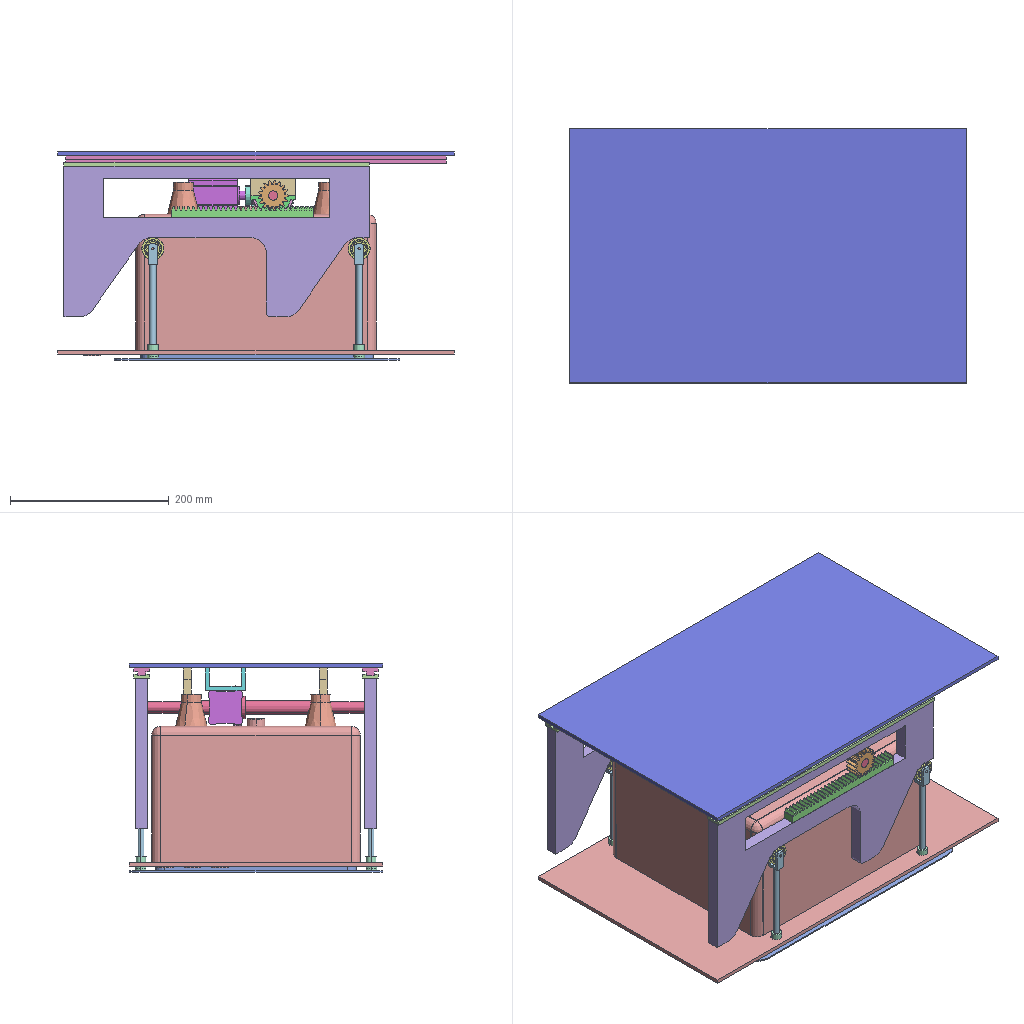Assembly | SolidWorks | 23 different items | 46 placed | box 500 x 320 x 263 mm
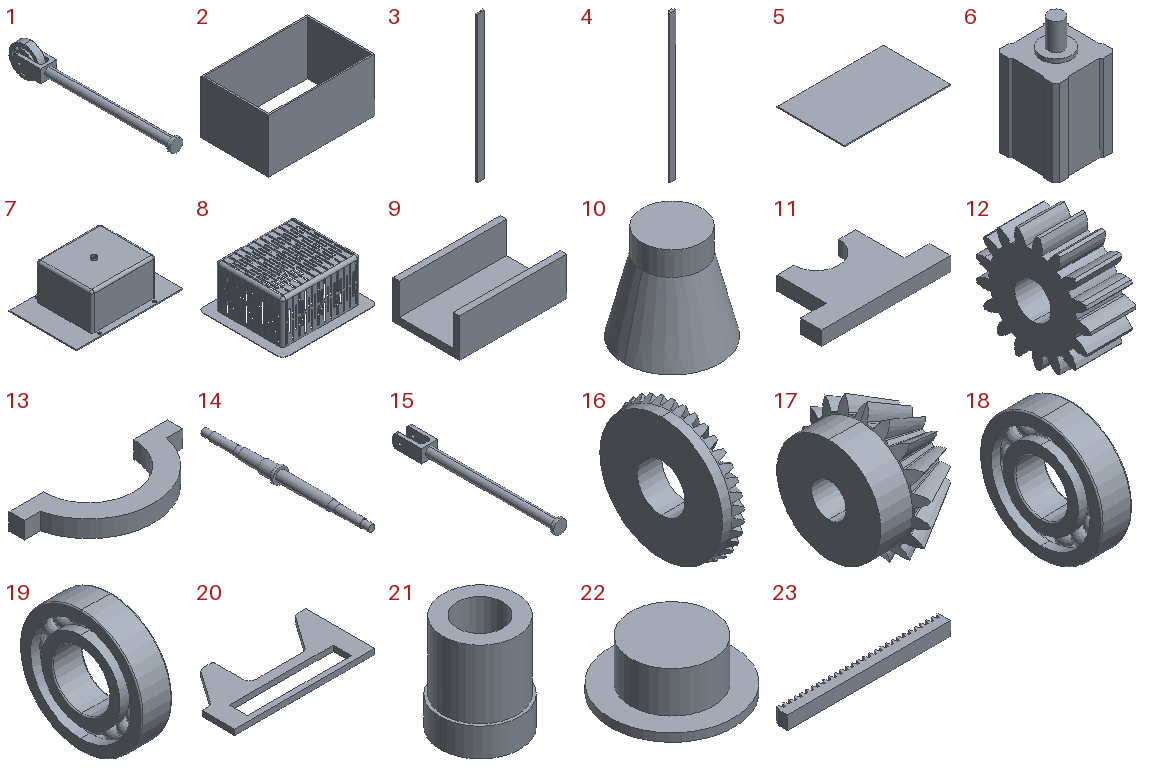Parts list (item | name | quantity | parent item | size | volume | features):
1 | (subassembly) | x4 | - | 15 x 153 x 28 mm | 10997 mm3 | -
2 | - | x1 | - | 500 x 320 x 252.7 mm | 3250733 mm3 | features Extrusion 1
3 | - | x2 | - | 20 x 5 x 385 mm | 30800 mm3 | features Extrusion 1
4 | - | x2 | - | 20 x 10 x 480 mm | 72000 mm3 | features Extrusion 1
5 | - | x1 | - | 500 x 320 x 5 mm | 800000 mm3 | features Extrusion 1
6 | - | x1 | - | 42.35 x 42.35 x 83.6 mm | 106285 mm3 | features ICE 5, CirPattern 1, Extrusion 1, RefAxis 1, Scale 1
7 | - | x1 | - | 500 x 320 x 188.5 mm | 804078 mm3 | features ICE 5, Fillet 2, Extrusion 1
8 | - | x1 | - | 360 x 320 x 163 mm | 306732 mm3 | features ICE 5, Fillet 3, Extrusion 1
9 | - | x1 | - | 80 x 50 x 28.83 mm | 39671 mm3 | features Extrusion 1, ICE 1
10 | - | x4 | - | 40 x 40 x 40 mm | 30238 mm3 | features Blend 1, ICE 1
11 | - | x2 | - | 92 x 50 x 10 mm | 29379 mm3 | features Extrusion 1
12 | - | x2 | - | 15 x 37.761 x 37.916 mm | 11362 mm3 | features Boss 3, Cut 3, CirPattern 2, Fillet 2, Revolution 1
13 | - | x2 | - | 56 x 22.979 x 6 mm | 2901 mm3 | features Extrusion 1
14 | - | x1 | - | 28 x 303 x 28 mm | 67053 mm3 | features Revolution 1
15 | - | x4 | in 1 | 15 x 145 x 12.163 mm | 8356 mm3 | features ICE 3, Fillet 2, Extrusion 1
16 | - | x1 | - | 12.396 x 54.775 x 54.775 mm | 16791 mm3 | features CirPattern 2, Cut 2, BlendCut 1, Boss 1, ICE 1, Revolution 1
17 | - | x1 | - | 19.27 x 30.102 x 30.566 mm | 6755 mm3 | features CirPattern 2, Cut 2, BlendCut 1, Boss 1, Revolution 1
18 | - | x4 | in 1 | 7 x 28 x 28 mm | 2641 mm3 | features Revolution 3, CirPattern 1, Fillet 1
19 | - | x2 | - | 8 x 32 x 32 mm | 3760 mm3 | features Revolution 3, CirPattern 1, Fillet 1
20 | - | x2 | - | 385 x 190 x 15 mm | 496112 mm3 | features Extrusion 1
21 | - | x4 | - | 14 x 14 x 17 mm | 1508 mm3 | features Extrusion 1, ICE 1
22 | - | x1 | - | 30 x 30 x 12 mm | 4555 mm3 | features Extrusion 1, ICE 1
23 | - | x2 | - | 180 x 14 x 15 mm | 31331 mm3 | features Cut 2, Extrusion 1, LPattern 1
Mates (type | each side: item.copy, entity, surface, feature):
In the top assembly
Concentric | 7.1 face cylinder Boss-Extrude3 | 22.1 face cylinder Boss-Extrude2
Coincident | 7.1 face plane Boss-Extrude3 | 22.1 face plane Boss-Extrude1
Coincident | 7.1 face plane Boss-Extrude1 | 8.1 face plane Boss-Extrude1
DistanceDim | 16.1 face plane Hub | 7.1 face plane Boss-Extrude2
Concentric | 16.1 face cylinder Cut-Extrude2 | 12.1 face cylinder Bore
Concentric | 16.1 face cylinder Cut-Extrude2 | 12.2 face cylinder Bore
DistanceDim | 12.1 face plane Base-Revolve | 7.1 face plane Boss-Extrude2
DistanceDim | 12.2 face plane Base-Revolve | 7.1 face plane Boss-Extrude2
Coincident | 12.1 face plane Base-Revolve | 20.1 face plane Boss-Extrude1
Parallel | 7.1 face plane Boss-Extrude3 | 20.1 face plane Boss-Extrude1
Coincident | 12.2 face plane Base-Revolve | 20.2 face plane Boss-Extrude1
Coincident | 20.1 face plane Boss-Extrude1 | 20.2 face plane Boss-Extrude1
Coincident | 20.1 face plane Boss-Extrude1 | 23.1 face plane Blank | 2 times
Concentric | 7.1 face cylinder Cut-Extrude1 | 15.1 face cylinder Boss-Extrude2
Concentric | 7.1 face cylinder Cut-Extrude1 | 15.2 face cylinder Boss-Extrude2
Parallel | 20.1 face plane Boss-Extrude1 | 15.1 face plane Boss-Extrude1
Coincident | 15.1 face plane Boss-Extrude1 | 15.2 face plane Boss-Extrude1
Concentric | 7.1 face cylinder Cut-Extrude1 | 15.3 face cylinder Boss-Extrude2
Parallel | 20.2 face plane Boss-Extrude1 | 15.4 face plane Boss-Extrude1
Parallel | 20.2 face plane Boss-Extrude1 | 15.3 face plane Boss-Extrude1
Coincident | 20.2 face plane Boss-Extrude1 | 23.2 face plane Blank | 2 times
Concentric | 17.1 face cylinder Bore | 6.1 face cylinder Boss-Extrude1
Concentric | 7.1 face cylinder Cut-Extrude1 | 21.1 face cylinder Boss-Extrude2
Coincident | 7.1 face plane Boss-Extrude1 | 21.1 face plane Boss-Extrude1
Concentric | 7.1 face cylinder Cut-Extrude1 | 21.2 face cylinder Boss-Extrude2
Coincident | 7.1 face plane Boss-Extrude1 | 21.2 face plane Boss-Extrude1
Concentric | 7.1 face cylinder Cut-Extrude1 | 21.3 face cylinder Boss-Extrude2
Coincident | 7.1 face plane Boss-Extrude1 | 21.3 face plane Boss-Extrude1
Concentric | 7.1 face cylinder Cut-Extrude1 | 21.4 face cylinder Boss-Extrude2
Coincident | 7.1 face plane Boss-Extrude1 | 21.4 face plane Boss-Extrude1
Coincident | 23.1 face plane Blank | 23.2 face plane Blank | 2 times
DistanceDim | 6.1 face plane Extrude1 | 17.1 face plane Hub
Parallel | 7.1 face plane Boss-Extrude2 | 6.1 face plane Extrude1
Coincident | 7.1 face plane Boss-Extrude1 | 2.1 face plane Boss-Extrude1 | 2 times
DistanceDim | 8.1 face plane Boss-Extrude2 | 7.1 face plane Boss-Extrude1
DistanceDim | 23.1 face plane Blank | 20.1 face plane Boss-Extrude1
Coincident | 10.1 face plane Boss-Extrude1 | 10.2 face plane Boss-Extrude1
Coincident | 7.1 face plane Boss-Extrude3 | 10.1 face plane Loft1
Coincident | 10.1 face plane Boss-Extrude1 | 10.3 face plane Boss-Extrude1
Coincident | 10.1 face plane Boss-Extrude1 | 10.4 face plane Boss-Extrude1
DistanceDim | 10.3 face cylinder Boss-Extrude1 | 7.1 face plane Boss-Extrude2 | 2 times
DistanceDim | 10.2 face cylinder Boss-Extrude1 | 7.1 face plane Boss-Extrude2 | 2 times
DistanceDim | 10.1 face cylinder Boss-Extrude1 | 7.1 face plane Boss-Extrude2 | 2 times
DistanceDim | 10.4 face cylinder Boss-Extrude1 | 7.1 face plane Boss-Extrude2 | 2 times
Coincident | 7.1 face plane Boss-Extrude1 | 5.1 face plane Boss-Extrude1 | 2 times
Coincident | 5.1 face plane Boss-Extrude1 | 4.1 face plane Boss-Extrude1
Coincident | 4.1 face plane Boss-Extrude1 | 4.2 face plane Boss-Extrude1 | 2 times
DistanceDim | 4.1 face plane Boss-Extrude1 | 20.2 face plane Boss-Extrude1
DistanceDim | 4.1 face plane Boss-Extrude1 | 5.1 face plane Boss-Extrude1
DistanceDim | 4.2 face plane Boss-Extrude1 | 20.1 face plane Boss-Extrude1
Coincident | 20.2 face plane Boss-Extrude1 | 3.1 face plane Boss-Extrude1 | 2 times
Coincident | 3.1 face plane Boss-Extrude1 | 4.1 face plane Boss-Extrude1 | 2 times
Coincident | 20.1 face plane Boss-Extrude1 | 3.2 face plane Boss-Extrude1
Coincident | 3.2 face plane Boss-Extrude1 | 4.2 face plane Boss-Extrude1
Coincident | 3.2 face plane Boss-Extrude1 | 20.1 face plane Boss-Extrude1
Parallel | 6.1 face plane Extrude1 | 5.1 face plane Boss-Extrude1
Coincident | 5.1 face plane Boss-Extrude1 | 9.1 face plane Boss-Extrude1
DistanceDim | 6.1 face plane Extrude1 | 9.1 face plane Boss-Extrude1 | 2 times
DistanceDim | 9.1 face plane Boss-Extrude1 | 6.1 face plane Extrude1
Coincident | 15.3 face plane Boss-Extrude3 | 15.4 face plane Boss-Extrude3
Coincident | 15.1 face plane Boss-Extrude3 | 15.4 face plane Boss-Extrude3
Coincident | 15.1 face plane Boss-Extrude3 | 15.2 face plane Boss-Extrude3
Coincident | 8.1 face plane Boss-Extrude1 | 15.2 face plane Boss-Extrude3
DistanceDim | 4.1 face plane Boss-Extrude1 | 21.3 face plane Boss-Extrude2
Tangent | 20.2 face surface:4009 Boss-Extrude1 | 18.1 face cylinder Revolve3
DistanceDim | 6.1 face cylinder Boss-Extrude1 | 16.1 face plane Hub
DistanceDim | 6.1 face plane Extrude1 | 5.1 face plane Boss-Extrude1
Concentric | 12.1 face cylinder Bore | 14.1 face cylinder Revolve1
Coincident | 12.1 face plane Base-Revolve | 14.1 face plane Revolve1
DistanceDim | 14.1 face cylinder Revolve1 | 5.1 face plane Boss-Extrude1
DistanceDim | 17.1 face plane Hub | 14.1 face cylinder Revolve1
Concentric | 14.1 face cylinder Revolve1 | 11.1 face cylinder Boss-Extrude1
Parallel | 5.1 face plane Boss-Extrude1 | 11.1 face plane Boss-Extrude1
Coincident | 14.1 face plane Revolve1 | 11.1 face plane Boss-Extrude1
Concentric | 14.1 face cylinder Revolve1 | 11.2 face cylinder Boss-Extrude1
Coincident | 14.1 face plane Revolve1 | 11.2 face plane Boss-Extrude1
Parallel | 5.1 face plane Boss-Extrude1 | 11.2 face plane Boss-Extrude1
Concentric | 14.1 face cylinder Revolve1 | 19.1 face cylinder Revolve2
Coincident | 11.2 face plane Boss-Extrude1 | 19.1 face plane Revolve3
Concentric | 14.1 face cylinder Revolve1 | 19.2 face cylinder Revolve2
Coincident | 11.1 face plane Boss-Extrude1 | 19.2 face plane Revolve3
Concentric | 19.1 face cylinder Revolve3 | 13.1 face cylinder Boss-Extrude1
Coincident | 11.2 face plane Boss-Extrude1 | 13.1 face plane Boss-Extrude1
DistanceDim | 13.1 face plane Boss-Extrude1 | 11.2 face plane Boss-Extrude1
Coincident | 11.1 face plane Boss-Extrude1 | 13.2 face plane Boss-Extrude1
Concentric | 19.2 face cylinder Revolve3 | 13.2 face cylinder Boss-Extrude1
DistanceDim | 13.2 face plane Boss-Extrude1 | 11.1 face plane Boss-Extrude1
Concentric | 15.4 face cylinder Boss-Extrude2 | 21.4 face cylinder Boss-Extrude2
In subassembly 1
Concentric | 15.5 face cylinder Cut-Extrude1 | 18.2 face cylinder Revolve2
DistanceDim | 18.2 face plane Revolve2 | 15.5 face plane Boss-Extrude1